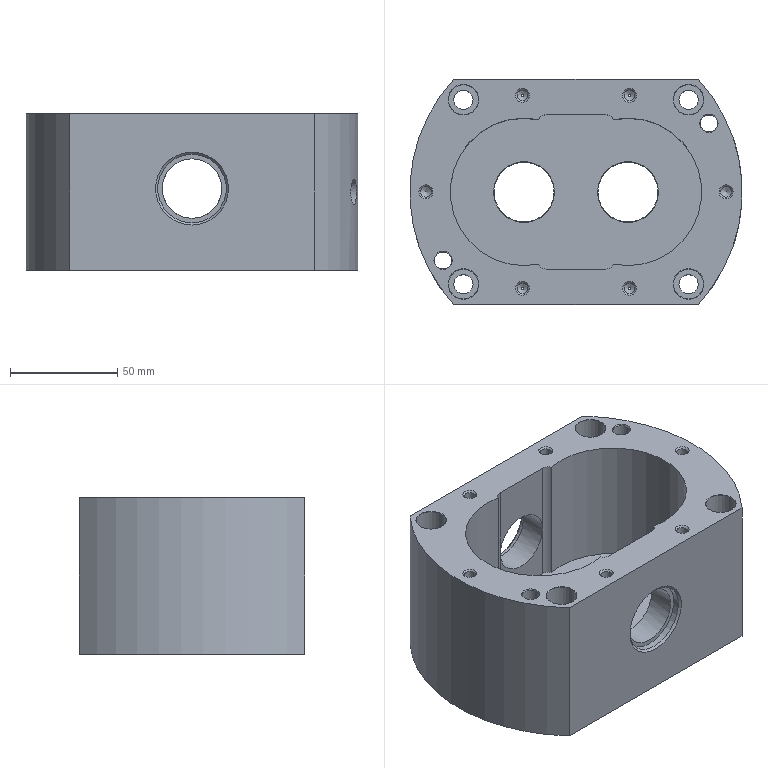NC program | NX | posted with a generic post | part box 155 x 105 x 73.2 mm
Whole program:
N10 G17 G21 G94 G90
(FLOOR_WALL , TOOL : D50)
N12 T02 M6
N14 G54
N16 G17 G0 G90 X-45.316 Y46.597 B0. C0. S1200 M3
N18 G43 Z30. H2
N20 Z2.654
N22 G94 G1 Z-0.346 F1000.
N24 X-42.316
N26 X42.316 F2000.
N28 Y9.999
N30 X-42.316
N32 Y-26.6
N34 X42.316
N36 X45.316
N38 Z2.654
N40 G0 Z30.
N42 X-48.333 Y46.597
N44 Z2.308
N46 G1 Z-0.692 F1000.
N48 X-45.333
N50 X45.333 F2000.
N52 Y9.999
N54 X-45.333
N56 Y-26.6
N58 X45.333
N60 X48.333
N62 Z2.308
N64 G0 Z30.
N66 X-50.64 Y46.597
N68 Z1.962
N70 G1 Z-1.038 F1000.
N72 X-47.64
N74 X47.64 F2000.
N76 Y9.999
N78 X-47.64
N80 Y-26.6
N82 X47.64
N84 X50.64
N86 Z1.962
N88 G0 Z30.
N90 X-52.579 Y46.597
N92 Z1.616
N94 G1 Z-1.384 F1000.
N96 X-49.579
N98 X49.579 F2000.
N100 Y9.999
N102 X-49.579
N104 Y-26.6
N106 X49.579
N108 X52.579
N110 Z1.616
N112 G0 Z30.
N114 X-54.281 Y46.597
N116 Z1.271
N118 G1 Z-1.729 F1000.
N120 X-51.281
N122 X51.281 F2000.
N124 Y9.999
N126 X-51.281
N128 Y-26.6
N130 X51.281
N132 X54.281
N134 Z1.271
N136 G0 Z30.
N138 X-55.815 Y46.597
N140 Z0.925
N142 G1 Z-2.075 F1000.
N144 X-52.815
N146 X52.815 F2000.
N148 Y9.999
N150 X-52.815
N152 Y-26.6
N154 X52.815
N156 X55.815
N158 Z0.925
N160 G0 Z30.
N162 X-57.22 Y46.597
N164 Z0.579
N166 G1 Z-2.421 F1000.
N168 X-54.22
N170 X54.22 F2000.
N172 Y9.999
N174 X-54.22
N176 Y-26.6
N178 X54.22
N180 X57.22
N182 Z0.579
N184 G0 Z30.
N186 X-58.524 Y46.597
N188 Z0.233
N190 G1 Z-2.767 F1000.
N192 X-55.524
N194 X55.524 F2000.
N196 Y9.999
N198 X-55.524
N200 Y-26.6
N202 X55.524
N204 X58.524
N206 Z0.233
N208 G0 Z30.
N210 X-59.744 Y46.597
N212 Z-0.113
N214 G1 Z-3.113 F1000.
N216 X-56.744
N218 X56.744 F2000.
N220 Y9.999
N222 X-56.744
N224 Y-26.6
N226 X56.744
N228 X59.744
N230 Z-0.113
N232 G0 Z30.
N234 X-60.894 Y46.597
N236 Z-0.459
N238 G1 Z-3.459 F1000.
N240 X-57.894
N242 X57.894 F2000.
N244 Y9.999
N246 X-57.894
N248 Y-26.6
N250 X57.894
N252 X60.894
N254 Z-0.459
N256 G0 Z30.
N258 X-61.984 Y46.597
N260 Z-0.804
N262 G1 Z-3.804 F1000.
N264 X-58.984
N266 X58.984 F2000.
N268 Y9.999
N270 X-58.984
N272 Y-26.6
N274 X58.984
N276 X61.984
N278 Z-0.804
N280 G0 Z30.
N282 X-63.021 Y46.597
N284 Z-1.15
N286 G1 Z-4.15 F1000.
N288 X-60.021
N290 X60.021 F2000.
N292 Y9.999
N294 X-60.021
N296 Y-26.6
N298 X60.021
N300 X63.021
N302 Z-1.15
N304 G0 Z30.
N306 X-64.013 Y46.597
N308 Z-1.496
N310 G1 Z-4.496 F1000.
N312 X-61.013
N314 X61.013 F2000.
N316 Y9.999
N318 X-61.013
N320 Y-26.6
N322 X61.013
N324 X64.013
N326 Z-1.496
N328 G0 Z30.
N330 X-64.964 Y46.597
N332 Z-1.842
N334 G1 Z-4.842 F1000.
N336 X-61.964
N338 X61.964 F2000.
N340 Y9.999
N342 X-61.964
N344 Y-26.6
N346 X61.964
N348 X64.964
N350 Z-1.842
N352 G0 Z30.
N354 X-65.878 Y46.597
N356 Z-2.188
N358 G1 Z-5.188 F1000.
N360 X-62.878
N362 X62.878 F2000.
N364 Y9.999
N366 X-62.878
N368 Y-26.6
N370 X62.878
N372 X65.878
N374 Z-2.188
N376 G0 Z30.
N378 X-66.759 Y46.597
N380 Z-2.534
N382 G1 Z-5.534 F1000.
N384 X-63.759
N386 X63.759 F2000.
N388 Y9.999
N390 X-63.759
N392 Y-26.6
N394 X63.759
N396 X66.759
N398 Z-2.534
N400 G0 Z30.
N402 X-67.61 Y46.597
N404 Z-2.879
N406 G1 Z-5.879 F1000.
N408 X-64.61
N410 X64.61 F2000.
N412 Y9.999
N414 X-64.61
N416 Y-26.6
N418 X64.61
N420 X67.61
N422 Z-2.879
N424 G0 Z30.
N426 X-68.433 Y46.597
N428 Z-3.225
N430 G1 Z-6.225 F1000.
N432 X-65.433
N434 X65.433 F2000.
N436 Y9.999
N438 X-65.433
N440 Y-26.6
N442 X65.433
N444 X68.433
N446 Z-3.225
N448 G0 Z30.
N450 X-69.23 Y46.597
N452 Z-3.571
N454 G1 Z-6.571 F1000.
N456 X-66.23
N458 X66.23 F2000.
N460 Y9.999
N462 X-66.23
N464 Y-26.6
N466 X66.23
N468 X69.23
N470 Z-3.571
N472 G0 Z30.
N474 X-70.004 Y46.597
N476 Z-3.917
N478 G1 Z-6.917 F1000.
N480 X-67.004
N482 X67.004 F2000.
N484 Y9.999
N486 X-67.004
N488 Y-26.6
N490 X67.004
N492 X70.004
N494 Z-3.917
N496 G0 Z30.
N498 X-70.756 Y46.597
N500 Z-4.263
N502 G1 Z-7.263 F1000.
N504 X-67.756
N506 X67.756 F2000.
N508 Y9.999
N510 X-67.756
N512 Y-26.6
N514 X67.756
N516 X70.756
N518 Z-4.263
N520 G0 Z30.
N522 X-71.488 Y46.597
N524 Z-4.609
N526 G1 Z-7.609 F1000.
N528 X-68.488
N530 X68.488 F2000.
N532 Y9.999
N534 X-68.488
N536 Y-26.6
N538 X68.488
N540 X71.488
N542 Z-4.609
N544 G0 Z30.
N546 X-72.2 Y46.597
N548 Z-4.954
N550 G1 Z-7.954 F1000.
N552 X-69.2
N554 X69.2 F2000.
N556 Y9.999
N558 X-69.2
N560 Y-26.6
N562 X69.2
N564 X72.2
N566 Z-4.954
N568 G0 Z30.
N570 X-72.895 Y46.597
N572 Z-5.3
N574 G1 Z-8.3 F1000.
N576 X-69.895
N578 X69.895 F2000.
N580 Y9.999
N582 X-69.895
N584 Y-26.6
N586 X69.895
N588 X72.895
N590 Z-5.3
N592 G0 Z30.
N594 X-73.572 Y46.597
N596 Z-5.646
N598 G1 Z-8.646 F1000.
N600 X-70.572
N602 X70.572 F2000.
N604 Y9.999
N606 X-70.572
N608 Y-26.6
N610 X70.572
N612 X73.572
N614 Z-5.646
N616 G0 Z30.
N618 X-74.234 Y46.597
N620 Z-5.992
N622 G1 Z-8.992 F1000.
N624 X-71.234
N626 X71.234 F2000.
N628 Y9.999
N630 X-71.234
N632 Y-26.6
N634 X71.234
N636 X74.234
N638 Z-5.992
N640 G0 Z30.
N642 X-74.88 Y46.597
N644 Z-6.338
N646 G1 Z-9.338 F1000.
N648 X-71.88
N650 X71.88 F2000.
N652 Y9.999
N654 X-71.88
N656 Y-26.6
N658 X71.88
N660 X74.88
N662 Z-6.338
N664 G0 Z30.
N666 X-75.512 Y46.597
N668 Z-6.684
N670 G1 Z-9.684 F1000.
N672 X-72.512
N674 X72.512 F2000.
N676 Y9.999
N678 X-72.512
N680 Y-26.6
N682 X72.512
N684 X75.512
N686 Z-6.684
N688 G0 Z30.
N690 X-76.131 Y46.597
N692 Z-7.029
N694 G1 Z-10.029 F1000.
N696 X-73.131
N698 X73.131 F2000.
N700 Y9.999
N702 X-73.131
N704 Y-26.6
N706 X73.131
N708 X76.131
N710 Z-7.029
N712 G0 Z30.
N714 X-76.736 Y46.597
N716 Z-7.375
N718 G1 Z-10.375 F1000.
N720 X-73.736
N722 X73.736 F2000.
N724 Y9.999
N726 X-73.736
N728 Y-26.6
N730 X73.736
N732 X76.736
N734 Z-7.375
N736 G0 Z30.
N738 X-77.33 Y46.597
N740 Z-7.721
N742 G1 Z-10.721 F1000.
N744 X-74.33
N746 X74.33 F2000.
N748 Y9.999
N750 X-74.33
N752 Y-26.6
N754 X74.33
N756 X77.33
N758 Z-7.721
N760 G0 Z30.
N762 X-77.911 Y46.597
N764 Z-8.067
N766 G1 Z-11.067 F1000.
N768 X-74.911
N770 X74.911 F2000.
N772 Y9.999
N774 X-74.911
N776 Y-26.6
N778 X74.911
N780 X77.911
N782 Z-8.067
N784 G0 Z30.
N786 X-78.481 Y46.597
N788 Z-8.413
N790 G1 Z-11.413 F1000.
N792 X-75.481
N794 X75.481 F2000.
N796 Y9.999
N798 X-75.481
N800 Y-26.6
N802 X75.481
N804 X78.481
N806 Z-8.413
N808 G0 Z30.
N810 X-79.04 Y46.597
N812 Z-8.758
N814 G1 Z-11.758 F1000.
N816 X-76.04
N818 X76.04 F2000.
N820 Y9.999
N822 X-76.04
N824 Y-26.6
N826 X76.04
N828 X79.04
N830 Z-8.758
N832 G0 Z30.
N834 X-79.589 Y46.597
N836 Z-9.104
N838 G1 Z-12.104 F1000.
N840 X-76.589
N842 X76.589 F2000.
N844 Y9.999
N846 X-76.589
N848 Y-26.6
N850 X76.589
N852 X79.589
N854 Z-9.104
N856 G0 Z30.
N858 X-80.128 Y46.597
N860 Z-9.45
N862 G1 Z-12.45 F1000.
N864 X-77.128
N866 X77.128 F2000.
N868 Y9.999
N870 X-77.128
N872 Y-26.6
N874 X77.128
N876 X80.128
N878 Z-9.45
N880 G0 Z30.
N882 X-80.657 Y46.597
N884 Z-9.796
N886 G1 Z-12.796 F1000.
N888 X-77.657
N890 X77.657 F2000.
N892 Y9.999
N894 X-77.657
N896 Y-26.6
N898 X77.657
N900 X80.657
N902 Z-9.796
N904 G0 Z30.
N906 X-81.177 Y46.597
N908 Z-10.142
N910 G1 Z-13.142 F1000.
N912 X-78.177
N914 X78.177 F2000.
N916 Y9.999
N918 X-78.177
N920 Y-26.6
N922 X78.177
N924 X81.177
N926 Z-10.142
N928 G0 Z30.
N930 X-81.688 Y46.597
N932 Z-10.488
N934 G1 Z-13.488 F1000.
N936 X-78.688
N938 X78.688 F2000.
N940 Y9.999
N942 X-78.688
N944 Y-26.6
N946 X78.688
N948 X81.688
N950 Z-10.488
N952 G0 Z30.
N954 X-82.191 Y46.597
N956 Z-10.833
N958 G1 Z-13.833 F1000.
N960 X-79.191
N962 X79.191 F2000.
N964 Y9.999
N966 X-79.191
N968 Y-26.6
N970 X79.191
N972 X82.191
N974 Z-10.833
N976 G0 Z30.
N978 X-82.685 Y46.597
N980 Z-11.179
N982 G1 Z-14.179 F1000.
N984 X-79.685
N986 X79.685 F2000.
N988 Y9.999
N990 X-79.685
N992 Y-26.6
N994 X79.685
N996 X82.685
N998 Z-11.179
N1000 G0 Z30.
N1002 X-83.171 Y46.597
N1004 Z-11.525
N1006 G1 Z-14.525 F1000.
N1008 X-80.171
N1010 X80.171 F2000.
N1012 Y9.999
N1014 X-80.171
N1016 Y-26.6
N1018 X80.171
N1020 X83.171
N1022 Z-11.525
N1024 G0 Z30.
N1026 X-83.649 Y46.597
N1028 Z-11.871
N1030 G1 Z-14.871 F1000.
N1032 X-80.649
N1034 X80.649 F2000.
N1036 Y9.999
N1038 X-80.649
N1040 Y-26.6
N1042 X80.649
N1044 X83.649
N1046 Z-11.871
N1048 G0 Z30.
N1050 X-84.12 Y46.597
N1052 Z-12.217
N1054 G1 Z-15.217 F1000.
N1056 X-81.12
N1058 X81.12 F2000.
N1060 Y9.999
N1062 X-81.12
N1064 Y-26.6
N1066 X81.12
N1068 X84.12
N1070 Z-12.217
N1072 G0 Z30.
N1074 X-84.583 Y46.597
N1076 Z-12.563
N1078 G1 Z-15.563 F1000.
N1080 X-81.583
N1082 X81.583 F2000.
N1084 Y9.999
N1086 X-81.583
N1088 Y-26.6
N1090 X81.583
N1092 X84.583
N1094 Z-12.563
N1096 G0 Z30.
N1098 X-85.04 Y46.597
N1100 Z-12.908
N1102 G1 Z-15.908 F1000.
N1104 X-82.04
N1106 X82.04 F2000.
N1108 Y9.999
N1110 X-82.04
N1112 Y-26.6
N1114 X82.04
N1116 X85.04
N1118 Z-12.908
N1120 G0 Z30.
N1122 X-85.489 Y46.597
N1124 Z-13.254
N1126 G1 Z-16.254 F1000.
N1128 X-82.489
N1130 X82.489 F2000.
N1132 Y9.999
N1134 X-82.489
N1136 Y-26.6
N1138 X82.489
N1140 X85.489
N1142 Z-13.254
N1144 G0 Z30.
N1146 X-85.932 Y46.597
N1148 Z-13.6
N1150 G1 Z-16.6 F1000.
N1152 X-82.932
N1154 X82.932 F2000.
N1156 Y9.999
N1158 X-82.932
N1160 Y-26.6
N1162 X82.932
N1164 X85.932
N1166 Z-13.6
N1168 G0 Z30.
N1170 X-86.368 Y46.597
N1172 Z-13.946
N1174 G1 Z-16.946 F1000.
N1176 X-83.368
N1178 X83.368 F2000.
N1180 Y9.999
N1182 X-83.368
N1184 Y-26.6
N1186 X83.368
N1188 X86.368
N1190 Z-13.946
N1192 G0 Z30.
N1194 X-86.798 Y46.597
N1196 Z-14.292
N1198 G1 Z-17.292 F1000.
N1200 X-83.798
N1202 X83.798 F2000.
N1204 Y9.999
N1206 X-83.798
N1208 Y-26.6
N1210 X83.798
N1212 X86.798
N1214 Z-14.292
N1216 G0 Z30.
N1218 X-87.221 Y46.597
N1220 Z-14.638
N1222 G1 Z-17.638 F1000.
N1224 X-84.221
N1226 X84.221 F2000.
N1228 Y9.999
N1230 X-84.221
N1232 Y-26.6
N1234 X84.221
N1236 X87.221
N1238 Z-14.638
N1240 G0 Z30.
N1242 X-87.639 Y46.597
N1244 Z-14.983
N1246 G1 Z-17.983 F1000.
N1248 X-84.639
N1250 X84.639 F2000.
N1252 Y9.999
N1254 X-84.639
N1256 Y-26.6
N1258 X84.639
N1260 X87.639
N1262 Z-14.983
N1264 G0 Z30.
N1266 X-88.051 Y46.597
N1268 Z-15.329
N1270 G1 Z-18.329 F1000.
N1272 X-85.051
N1274 X85.051 F2000.
N1276 Y9.999
N1278 X-85.051
N1280 Y-26.6
N1282 X85.051
N1284 X88.051
N1286 Z-15.329
N1288 G0 Z30.
N1290 X-88.457 Y46.597
N1292 Z-15.675
N1294 G1 Z-18.675 F1000.
N1296 X-85.457
N1298 X85.457 F2000.
N1300 Y9.999
N1302 X-85.457
N1304 Y-26.6
N1306 X85.457
N1308 X88.457
N1310 Z-15.675
N1312 G0 Z30.
N1314 X-88.857 Y46.597
N1316 Z-16.021
N1318 G1 Z-19.021 F1000.
N1320 X-85.857
N1322 X85.857 F2000.
N1324 Y9.999
N1326 X-85.857
N1328 Y-26.6
N1330 X85.857
N1332 X88.857
N1334 Z-16.021
N1336 G0 Z30.
N1338 X-89.252 Y46.597
N1340 Z-16.367
N1342 G1 Z-19.367 F1000.
N1344 X-86.252
N1346 X86.252 F2000.
N1348 Y9.999
N1350 X-86.252
N1352 Y-26.6
N1354 X86.252
N1356 X89.252
N1358 Z-16.367
N1360 G0 Z30.
N1362 X-89.642 Y46.597
N1364 Z-16.713
N1366 G1 Z-19.713 F1000.
N1368 X-86.642
N1370 X86.642 F2000.
N1372 Y9.999
N1374 X-86.642
N1376 Y-26.6
N1378 X86.642
N1380 X89.642
N1382 Z-16.713
N1384 G0 Z30.
N1386 X-90.026 Y46.597
N1388 Z-17.058
N1390 G1 Z-20.058 F1000.
N1392 X-87.026
N1394 X87.026 F2000.
N1396 Y9.999
N1398 X-87.026
N1400 Y-26.6
N1402 X87.026
N1404 X90.026
N1406 Z-17.058
N1408 G0 Z30.
N1410 X-90.405 Y46.597
N1412 Z-17.404
N1414 G1 Z-20.404 F1000.
N1416 X-87.405
N1418 X87.405 F2000.
N1420 Y9.999
N1422 X-87.405
N1424 Y-26.6
N1426 X87.405
N1428 X90.405
N1430 Z-17.404
N1432 G0 Z30.
N1434 X-90.78 Y46.597
N1436 Z-17.75
N1438 G1 Z-20.75 F1000.
N1440 X-87.78
N1442 X87.78 F2000.
N1444 Y9.999
N1446 X-87.78
N1448 Y-26.6
N1450 X87.78
N1452 X90.78
N1454 Z-17.75
N1456 G0 Z30.
N1458 X-91.149 Y46.597
N1460 Z-18.096
N1462 G1 Z-21.096 F1000.
N1464 X-88.149
N1466 X88.149 F2000.
N1468 Y9.999
N1470 X-88.149
N1472 Y-26.6
N1474 X88.149
N1476 X91.149
N1478 Z-18.096
N1480 G0 Z30.
N1482 X-91.514 Y46.597
N1484 Z-18.442
N1486 G1 Z-21.442 F1000.
N1488 X-88.514
N1490 X88.514 F2000.
N1492 Y9.999
N1494 X-88.514
N1496 Y-26.6
N1498 X88.514
N1500 X91.514
N1502 Z-18.442
N1504 G0 Z30.
N1506 X-91.874 Y46.597
N1508 Z-18.788
N1510 G1 Z-21.788 F1000.
N1512 X-88.874
N1514 X88.874 F2000.
N1516 Y9.999
N1518 X-88.874
N1520 Y-26.6
N1522 X88.874
N1524 X91.874
N1526 Z-18.788
N1528 G0 Z30.
N1530 X-92.229 Y46.597
N1532 Z-19.133
N1534 G1 Z-22.133 F1000.
N1536 X-89.229
N1538 X89.229 F2000.
N1540 Y9.999
N1542 X-89.229
N1544 Y-26.6
N1546 X89.229
N1548 X92.229
N1550 Z-19.133
N1552 G0 Z30.
N1554 X-92.58 Y46.597
N1556 Z-19.479
N1558 G1 Z-22.479 F1000.
N1560 X-89.58
N1562 X89.58 F2000.
N1564 Y9.999
N1566 X-89.58
N1568 Y-26.6
N1570 X89.58
N1572 X92.58
N1574 Z-19.479
N1576 G0 Z30.
N1578 X-92.926 Y46.597
N1580 Z-19.825
N1582 G1 Z-22.825 F1000.
N1584 X-89.926
N1586 X89.926 F2000.
N1588 Y9.999
N1590 X-89.926
N1592 Y-26.6
N1594 X89.926
N1596 X92.926
N1598 Z-19.825
N1600 G0 Z30.
N1602 X-93.268 Y46.597
N1604 Z-20.171
N1606 G1 Z-23.171 F1000.
N1608 X-90.268
N1610 X90.268 F2000.
N1612 Y9.999
N1614 X-90.268
N1616 Y-26.6
N1618 X90.268
N1620 X93.268
N1622 Z-20.171
N1624 G0 Z30.
N1626 X-93.606 Y46.597
N1628 Z-20.517
N1630 G1 Z-23.517 F1000.
N1632 X-90.606
N1634 X90.606 F2000.
N1636 Y9.999
N1638 X-90.606
N1640 Y-26.6
N1642 X90.606
N1644 X93.606
N1646 Z-20.517
N1648 G0 Z30.
N1650 X-93.94 Y46.597
N1652 Z-20.863
N1654 G1 Z-23.863 F1000.
N1656 X-90.94
N1658 X90.94 F2000.
N1660 Y9.999
N1662 X-90.94
N1664 Y-26.6
N1666 X90.94
N1668 X93.94
N1670 Z-20.863
N1672 G0 Z30.
N1674 X-94.269 Y46.597
N1676 Z-21.208
N1678 G1 Z-24.208 F1000.
N1680 X-91.269
N1682 X91.269 F2000.
N1684 Y9.999
N1686 X-91.269
N1688 Y-26.6
N1690 X91.269
N1692 X94.269
N1694 Z-21.208
N1696 G0 Z30.
N1698 X-94.595 Y46.597
N1700 Z-21.554
N1702 G1 Z-24.554 F1000.
N1704 X-91.595
N1706 X91.595 F2000.
N1708 Y9.999
N1710 X-91.595
N1712 Y-26.6
N1714 X91.595
N1716 X94.595
N1718 Z-21.554
N1720 G0 Z30.
N1722 X-94.917 Y46.597
N1724 Z-21.9
N1726 G1 Z-24.9 F1000.
N1728 X-91.917
N1730 X91.917 F2000.
N1732 Y9.999
N1734 X-91.917
N1736 Y-26.6
N1738 X91.917
N1740 X94.917
N1742 Z-21.9
N1744 G0 Z30.
(FLOOR_WALL_COPY , TOOL : D50)
N1746 X-95.009 Y46.597 S2500
N1748 Z-22.
N1750 G1 Z-25. F1000.
N1752 X-92.009
N1754 X92.009
N1756 Y9.999
N1758 X-92.009
N1760 Y-26.6
N1762 X92.009
N1764 X95.009
N1766 Z-22.
N1768 G0 Z30.
N1770 M5
(HOLE_MILLING , TOOL : D10)
N1772 T10 M6
N1774 G54
N1776 G17 G0 G90 X0. Y-1.6 B0. C0. S3000 M3
N1778 G43 Z30. H10
N1780 Z-24.5
N1782 G94 G3 X-1.25 Y-0.35 R1.25 F2200.
N1784 X-2.5 Y-1.6 R1.25
N1786 X-2.5 Y-1.6 Z-24.72 I2.5 J0.
N1788 X-2.5 Y-1.6 Z-24.94 I2.5 J0.
N1790 X-2.5 Y-1.6 Z-25.16 I2.5 J0.
N1792 X-2.5 Y-1.6 Z-25.38 I2.5 J0.
N1794 X-2.5 Y-1.6 Z-25.6 I2.5 J0.
N1796 X-2.5 Y-1.6 Z-25.82 I2.5 J0.
N1798 X-2.5 Y-1.6 Z-26.04 I2.5 J0.
N1800 X-2.5 Y-1.6 Z-26.26 I2.5 J0.
N1802 X-2.5 Y-1.6 Z-26.48 I2.5 J0.
N1804 X-2.5 Y-1.6 Z-26.7 I2.5 J0.
N1806 X-2.5 Y-1.6 Z-26.92 I2.5 J0.
N1808 X-2.5 Y-1.6 Z-27.14 I2.5 J0.
N1810 X-2.5 Y-1.6 Z-27.36 I2.5 J0.
N1812 X-2.5 Y-1.6 Z-27.58 I2.5 J0.
N1814 X-2.5 Y-1.6 Z-27.8 I2.5 J0.
N1816 X-2.5 Y-1.6 Z-28.02 I2.5 J0.
N1818 X-2.5 Y-1.6 Z-28.24 I2.5 J0.
N1820 X-2.5 Y-1.6 Z-28.46 I2.5 J0.
N1822 X-2.5 Y-1.6 Z-28.68 I2.5 J0.
N1824 X-2.5 Y-1.6 Z-28.9 I2.5 J0.
N1826 X2.399 Y-2.304 Z-29. R2.5
N1828 X0.711 Y0.836 R2.538
N1830 X-2.483 Y-0.8 R2.572
N1832 X-0.863 Y-4.12 R2.629
N1834 X2.565 Y-2.5 R2.698
N1836 X0.966 Y0.999 R2.738
N1838 X-2.643 Y-0.595 R2.807
N1840 X-1.073 Y-4.274 R2.847
N1842 X2.716 Y-2.715 R2.916
N1844 X1.185 Y1.146 R2.956
N1846 X-2.786 Y-0.371 R3.025
N1848 X-1.301 Y-4.414 R3.065
N1850 X2.852 Y-2.948 R3.135
N1852 X1.422 Y1.277 R3.174
N1854 X-2.914 Y-0.13 R3.244
N1856 X-1.546 Y-4.536 R3.283
N1858 X2.971 Y-3.197 R3.353
N1860 X1.675 Y1.39 R3.392
N1862 X-3.023 Y0.128 R3.462
N1864 X-1.807 Y-4.64 R3.501
N1866 X3.07 Y-3.462 R3.571
N1868 X1.943 Y1.484 R3.611
N1870 X-3.113 Y0.4 R3.68
N1872 X-2.083 Y-4.724 R3.72
N1874 X3.15 Y-3.742 R3.789
N1876 X2.226 Y1.558 R3.829
N1878 X-3.182 Y0.687 R3.898
N1880 X-2.372 Y-4.787 R3.938
N1882 X3.208 Y-4.034 R4.007
N1884 X2.521 Y1.61 R4.047
N1886 X-3.229 Y0.985 R4.116
N1888 X-2.673 Y-4.828 R4.156
N1890 X3.244 Y-4.338 R4.226
N1892 X2.827 Y1.64 R4.265
N1894 X-3.254 Y1.294 R4.335
N1896 X-2.984 Y-4.846 R4.374
N1898 X3.257 Y-4.652 R4.444
N1900 X3.143 Y1.646 R4.483
N1902 X-3.254 Y1.612 R4.553
N1904 X-3.303 Y-4.84 R4.592
N1906 X3.245 Y-4.974 R4.662
N1908 X3.466 Y1.628 R4.701
N1910 X-3.23 Y1.938 R4.771
N1912 X-3.63 Y-4.809 R4.811
N1914 X3.209 Y-5.303 R4.88
N1916 X3.796 Y1.584 R4.92
N1918 X-3.181 Y2.27 R4.989
N1920 X-3.962 Y-4.753 R5.029
N1922 X3.146 Y-5.637 R5.098
N1924 X4.13 Y1.515 R5.138
N1926 X-3.105 Y2.605 R5.207
N1928 X-4.298 Y-4.67 R5.247
N1930 X3.058 Y-5.974 R5.316
N1932 X4.466 Y1.419 R5.356
N1934 X-3.003 Y2.942 R5.426
N1936 X-4.635 Y-4.561 R5.465
N1938 X2.942 Y-6.311 R5.535
N1940 X4.803 Y1.296 R5.574
N1942 X-2.874 Y3.28 R5.644
N1944 X-4.972 Y-4.425 R5.683
N1946 X2.799 Y-6.649 R5.753
N1948 X5.139 Y1.146 R5.792
N1950 X-2.718 Y3.616 R5.862
N1952 X-5.306 Y-4.261 R5.902
N1954 X2.629 Y-6.983 R5.971
N1956 X5.472 Y0.969 R6.011
N1958 X-2.534 Y3.949 R6.08
N1960 X-5.637 Y-4.07 R6.12
N1962 X2.432 Y-7.313 R6.189
N1964 X5.8 Y0.764 R6.229
N1966 X-2.323 Y4.276 R6.298
N1968 X-5.962 Y-3.852 R6.338
N1970 X2.207 Y-7.636 R6.407
N1972 X6.121 Y0.533 R6.447
N1974 X-2.084 Y4.595 R6.516
N1976 X-6.278 Y-3.606 R6.556
N1978 X1.955 Y-7.951 R6.626
N1980 X6.433 Y0.273 R6.665
N1982 X-1.819 Y4.905 R6.735
N1984 X-6.585 Y-3.334 R6.774
N1986 X1.676 Y-8.256 R6.844
N1988 X6.734 Y-0.012 R6.883
N1990 X-1.526 Y5.204 R6.953
N1992 X-6.879 Y-3.035 R6.992
N1994 X1.37 Y-8.548 R7.062
N1996 X7.021 Y-0.325 R7.102
N1998 X-1.208 Y5.489 R7.171
N2000 X-7.16 Y-2.71 R7.211
N2002 X1.039 Y-8.826 R7.28
N2004 X7.295 Y-0.663 R7.32
N2006 X-0.864 Y5.759 R7.389
N2008 X-7.425 Y-2.359 R7.429
N2010 X0.682 Y-9.087 R7.498
N2012 X7.551 Y-1.025 R7.538
N2014 X-0.495 Y6.011 R7.607
N2016 X-7.672 Y-1.984 R7.647
N2018 X0.301 Y-9.33 R7.716
N2020 X7.789 Y-1.413 R7.756
N2022 X-0.102 Y6.245 R7.826
N2024 X-7.9 Y-1.585 R7.865
N2026 X-0.103 Y-9.554 R7.935
N2028 X8.006 Y-1.823 R7.974
N2030 X0.314 Y6.458 R8.044
N2032 X-8.106 Y-1.164 R8.083
N2034 X-0.53 Y-9.756 R8.153
N2036 X8.201 Y-2.255 R8.192
N2038 X0.752 Y6.648 R8.262
N2040 X-8.29 Y-0.721 R8.302
N2042 X-0.978 Y-9.934 R8.371
N2044 X8.372 Y-2.708 R8.411
N2046 X1.21 Y6.813 R8.48
N2048 X-8.449 Y-0.258 R8.52
N2050 X-1.446 Y-10.087 R8.589
N2052 X8.518 Y-3.18 R8.629
N2054 X1.687 Y6.953 R8.698
N2056 X-8.581 Y0.224 R8.738
N2058 X-1.932 Y-10.213 R8.807
N2060 X8.637 Y-3.671 R8.847
N2062 X2.182 Y7.066 R8.917
N2064 X-8.686 Y0.722 R8.956
N2066 X-2.436 Y-10.311 R9.026
N2068 X8.727 Y-4.178 R9.065
N2070 X2.693 Y7.15 R9.135
N2072 X-8.761 Y1.237 R9.174
N2074 X-2.954 Y-10.38 R9.244
N2076 X8.787 Y-4.7 R9.283
N2078 X3.218 Y7.203 R9.353
N2080 X-8.806 Y1.766 R9.392
N2082 X-3.486 Y-10.418 R9.462
N2084 X8.817 Y-5.234 R9.502
N2086 X3.756 Y7.225 R9.571
N2088 X-8.819 Y2.306 R9.611
N2090 X-4.03 Y-10.423 R9.68
N2092 X8.813 Y-5.78 R9.72
N2094 X4.305 Y7.214 R9.789
N2096 X-8.799 Y2.857 R9.829
N2098 X-4.583 Y-10.396 R9.898
N2100 X8.777 Y-6.335 R9.938
N2102 X4.863 Y7.169 R10.007
N2104 X-8.745 Y3.416 R10.047
N2106 X-5.144 Y-10.334 R10.117
N2108 X8.706 Y-6.898 R10.156
N2110 X5.427 Y7.09 R10.226
N2112 X-8.657 Y3.981 R10.265
N2114 X-5.711 Y-10.237 R10.335
N2116 X8.599 Y-7.465 R10.374
N2118 X5.996 Y6.976 R10.444
N2120 X-8.533 Y4.55 R10.483
N2122 X-6.281 Y-10.105 R10.553
N2124 X8.457 Y-8.036 R10.592
N2126 X6.567 Y6.825 R10.662
N2128 X-8.372 Y5.121 R10.702
N2130 X-6.852 Y-9.936 R10.771
N2132 X8.325 Y-8.578 R10.828
N2134 X7.138 Y6.638 R10.862
N2136 X-8.238 Y5.538 R10.9
N2138 X7.138 Y6.638 R-10.9
N2140 X-0.55 Y6.088 R5.45
N2142 X0. Y-1.6 R5.45
N2144 G0 Z30.
(HOLE_MILLING_COPY , TOOL : D10)
N2146 Z-28.5
N2148 G3 X-1.25 Y-0.35 R1.25
N2150 X-2.5 Y-1.6 R1.25
N2152 X-2.5 Y-1.6 Z-28.72 I2.5 J0.
N2154 X-2.5 Y-1.6 Z-28.94 I2.5 J0.
N2156 X-2.5 Y-1.6 Z-29.16 I2.5 J0.
N2158 X-2.5 Y-1.6 Z-29.38 I2.5 J0.
N2160 X-2.5 Y-1.6 Z-29.6 I2.5 J0.
N2162 X-2.5 Y-1.6 Z-29.82 I2.5 J0.
N2164 X-2.5 Y-1.6 Z-30.04 I2.5 J0.
N2166 X-2.5 Y-1.6 Z-30.26 I2.5 J0.
N2168 X-2.5 Y-1.6 Z-30.48 I2.5 J0.
N2170 X-2.5 Y-1.6 Z-30.7 I2.5 J0.
N2172 X-2.5 Y-1.6 Z-30.92 I2.5 J0.
N2174 X-2.5 Y-1.6 Z-31.14 I2.5 J0.
N2176 X-2.5 Y-1.6 Z-31.36 I2.5 J0.
N2178 X-2.5 Y-1.6 Z-31.58 I2.5 J0.
N2180 X-2.5 Y-1.6 Z-31.8 I2.5 J0.
N2182 X-2.5 Y-1.6 Z-32.02 I2.5 J0.
N2184 X-2.5 Y-1.6 Z-32.24 I2.5 J0.
N2186 X-2.5 Y-1.6 Z-32.46 I2.5 J0.
N2188 X-2.5 Y-1.6 Z-32.68 I2.5 J0.
N2190 X-2.5 Y-1.6 Z-32.9 I2.5 J0.
N2192 X-2.5 Y-1.6 Z-33.12 I2.5 J0.
N2194 X-2.5 Y-1.6 Z-33.34 I2.5 J0.
N2196 X-2.5 Y-1.6 Z-33.56 I2.5 J0.
N2198 X-2.5 Y-1.6 Z-33.78 I2.5 J0.
N2200 X-2.5 Y-1.6 Z-34. I2.5 J0.
N2202 X-2.5 Y-1.6 Z-34.22 I2.5 J0.
N2204 X-2.5 Y-1.6 Z-34.44 I2.5 J0.
N2206 X-2.5 Y-1.6 Z-34.66 I2.5 J0.
N2208 X-2.5 Y-1.6 Z-34.88 I2.5 J0.
N2210 X-2.5 Y-1.6 Z-35.1 I2.5 J0.
N2212 X-2.5 Y-1.6 Z-35.32 I2.5 J0.
N2214 X-2.5 Y-1.6 Z-35.54 I2.5 J0.
N2216 X-2.5 Y-1.6 Z-35.76 I2.5 J0.
N2218 X-2.5 Y-1.6 Z-35.98 I2.5 J0.
N2220 X-2.5 Y-1.6 Z-36.2 I2.5 J0.
N2222 X-2.5 Y-1.6 Z-36.42 I2.5 J0.
N2224 X-2.5 Y-1.6 Z-36.64 I2.5 J0.
N2226 X-2.5 Y-1.6 Z-36.86 I2.5 J0.
N2228 X-2.5 Y-1.6 Z-37.08 I2.5 J0.
N2230 X-2.5 Y-1.6 Z-37.3 I2.5 J0.
N2232 X-2.5 Y-1.6 Z-37.52 I2.5 J0.
N2234 X-2.5 Y-1.6 Z-37.74 I2.5 J0.
N2236 X-2.5 Y-1.6 Z-37.96 I2.5 J0.
N2238 X-2.5 Y-1.6 Z-38.18 I2.5 J0.
N2240 X-2.5 Y-1.6 Z-38.4 I2.5 J0.
N2242 X-2.5 Y-1.6 Z-38.62 I2.5 J0.
N2244 X-2.5 Y-1.6 Z-38.84 I2.5 J0.
N2246 X-2.5 Y-1.6 Z-39.06 I2.5 J0.
N2248 X-2.5 Y-1.6 Z-39.28 I2.5 J0.
N2250 X-2.5 Y-1.6 Z-39.5 I2.5 J0.
N2252 X-2.5 Y-1.6 Z-39.72 I2.5 J0.
N2254 X-2.5 Y-1.6 Z-39.94 I2.5 J0.
N2256 X-2.5 Y-1.6 Z-40.16 I2.5 J0.
N2258 X-2.5 Y-1.6 Z-40.38 I2.5 J0.
N2260 X-2.5 Y-1.6 Z-40.6 I2.5 J0.
N2262 X-2.5 Y-1.6 Z-40.82 I2.5 J0.
N2264 X-2.5 Y-1.6 Z-41.04 I2.5 J0.
N2266 X-2.5 Y-1.6 Z-41.26 I2.5 J0.
N2268 X-2.5 Y-1.6 Z-41.48 I2.5 J0.
N2270 X-2.5 Y-1.6 Z-41.7 I2.5 J0.
N2272 X-2.5 Y-1.6 Z-41.92 I2.5 J0.
N2274 X1.637 Y-3.489 Z-42. R2.5
N2276 X1.893 Y0.086 R2.534
N2278 X-1.703 Y0.365 R2.566
N2280 X-2.012 Y-3.325 R2.618
N2282 X1.768 Y-3.641 R2.682
N2284 X2.087 Y0.19 R2.718
N2286 X-1.834 Y0.516 R2.782
N2288 X-2.163 Y-3.456 R2.818
N2290 X1.899 Y-3.792 R2.882
N2292 X2.238 Y0.321 R2.918
N2294 X-1.965 Y0.667 R2.982
N2296 X-2.314 Y-3.587 R3.018
N2298 X2.03 Y-3.943 R3.082
N2300 X2.389 Y0.452 R3.118
N2302 X-2.096 Y0.818 R3.182
N2304 X-2.465 Y-3.718 R3.218
N2306 X2.161 Y-4.094 R3.282
N2308 X2.541 Y0.583 R3.318
N2310 X-2.227 Y0.97 R3.382
N2312 X-2.616 Y-3.849 R3.418
N2314 X2.292 Y-4.245 R3.482
N2316 X2.692 Y0.714 R3.518
N2318 X-2.357 Y1.121 R3.582
N2320 X-2.767 Y-3.98 R3.618
N2322 X2.423 Y-4.396 R3.682
N2324 X2.843 Y0.845 R3.718
N2326 X-2.488 Y1.272 R3.782
N2328 X-2.919 Y-4.111 R3.818
N2330 X2.554 Y-4.547 R3.882
N2332 X2.994 Y0.976 R3.918
N2334 X-2.619 Y1.423 R3.982
N2336 X-3.07 Y-4.242 R4.018
N2338 X2.685 Y-4.699 R4.082
N2340 X3.145 Y1.107 R4.118
N2342 X-2.75 Y1.574 R4.182
N2344 X-3.221 Y-4.373 R4.218
N2346 X2.816 Y-4.85 R4.282
N2348 X3.296 Y1.238 R4.318
N2350 X-2.881 Y1.725 R4.382
N2352 X-3.372 Y-4.504 R4.418
N2354 X2.947 Y-5.001 R4.482
N2356 X3.448 Y1.369 R4.518
N2358 X-3.012 Y1.876 R4.582
N2360 X-3.523 Y-4.635 R4.618
N2362 X3.078 Y-5.152 R4.682
N2364 X3.599 Y1.5 R4.718
N2366 X-3.143 Y2.028 R4.782
N2368 X-3.674 Y-4.766 R4.818
N2370 X3.209 Y-5.303 R4.882
N2372 X3.75 Y1.631 R4.918
N2374 X-3.274 Y2.179 R4.982
N2376 X-3.825 Y-4.897 R5.018
N2378 X3.34 Y-5.454 R5.082
N2380 X3.901 Y1.762 R5.118
N2382 X-3.405 Y2.33 R5.182
N2384 X-3.977 Y-5.028 R5.218
N2386 X3.471 Y-5.605 R5.282
N2388 X4.052 Y1.893 R5.318
N2390 X-3.536 Y2.481 R5.382
N2392 X-4.128 Y-5.159 R5.418
N2394 X3.602 Y-5.757 R5.482
N2396 X4.203 Y2.024 R5.518
N2398 X-3.667 Y2.632 R5.582
N2400 X-4.279 Y-5.29 R5.618
N2402 X3.733 Y-5.908 R5.682
N2404 X4.354 Y2.155 R5.718
N2406 X-3.798 Y2.783 R5.782
N2408 X-4.43 Y-5.421 R5.818
N2410 X3.864 Y-6.059 R5.882
N2412 X4.506 Y2.286 R5.918
N2414 X-3.929 Y2.934 R5.982
N2416 X-4.581 Y-5.552 R6.018
N2418 X3.995 Y-6.21 R6.082
N2420 X4.657 Y2.417 R6.118
N2422 X-4.06 Y3.086 R6.182
N2424 X-4.732 Y-5.683 R6.218
N2426 X4.126 Y-6.361 R6.282
N2428 X4.808 Y2.548 R6.318
N2430 X-4.191 Y3.237 R6.382
N2432 X-4.883 Y-5.813 R6.418
N2434 X4.257 Y-6.512 R6.482
N2436 X4.959 Y2.679 R6.518
N2438 X-4.322 Y3.388 R6.582
N2440 X-5.035 Y-5.944 R6.618
N2442 X4.388 Y-6.664 R6.682
N2444 X5.11 Y2.81 R6.718
N2446 X-4.453 Y3.539 R6.782
N2448 X-5.186 Y-6.075 R6.818
N2450 X4.519 Y-6.815 R6.882
N2452 X5.261 Y2.941 R6.918
N2454 X-4.584 Y3.69 R6.982
N2456 X-5.337 Y-6.206 R7.018
N2458 X4.65 Y-6.966 R7.082
N2460 X5.413 Y3.072 R7.118
N2462 X-4.715 Y3.841 R7.182
N2464 X-5.488 Y-6.337 R7.218
N2466 X4.78 Y-7.117 R7.282
N2468 X5.564 Y3.203 R7.318
N2470 X-4.846 Y3.993 R7.382
N2472 X-5.639 Y-6.468 R7.418
N2474 X4.911 Y-7.268 R7.482
N2476 X5.715 Y3.334 R7.518
N2478 X-4.977 Y4.144 R7.582
N2480 X-5.79 Y-6.599 R7.618
N2482 X5.042 Y-7.419 R7.682
N2484 X5.866 Y3.465 R7.718
N2486 X-5.108 Y4.295 R7.782
N2488 X-5.942 Y-6.73 R7.818
N2490 X5.173 Y-7.57 R7.882
N2492 X6.017 Y3.596 R7.918
N2494 X-5.239 Y4.446 R7.982
N2496 X-6.093 Y-6.861 R8.018
N2498 X5.304 Y-7.722 R8.082
N2500 X6.168 Y3.727 R8.118
N2502 X-5.37 Y4.597 R8.182
N2504 X-6.244 Y-6.992 R8.218
N2506 X5.435 Y-7.873 R8.282
N2508 X6.319 Y3.858 R8.318
N2510 X-5.501 Y4.748 R8.382
N2512 X-6.395 Y-7.123 R8.418
N2514 X5.566 Y-8.024 R8.482
N2516 X6.471 Y3.989 R8.518
N2518 X-5.632 Y4.899 R8.582
N2520 X-6.546 Y-7.254 R8.618
N2522 X5.697 Y-8.175 R8.682
N2524 X6.603 Y4.166 R8.734
N2526 X-5.763 Y5.051 R8.766
N2528 X-6.651 Y-7.363 R8.8
N2530 X-5.763 Y5.051 R-8.8
N2532 X-6.207 Y-1.156 R4.4
N2534 X0. Y-1.6 R4.4
N2536 G0 Z30.
N2538 M5
(HOLE_MILLING_COPY_1 , TOOL : D10JING)
N2540 T11 M6
N2542 G54
N2544 G17 G0 G90 X0. Y-1.6 B0. C0. S5000 M3
N2546 G43 Z30. H11
N2548 Z-29.
N2550 G94 G1 X-7.486 Y0.924 F1000.
N2552 G3 X-11. Y-1.6 R2.663
N2554 X0. Y-12.6 R11.
N2556 X-11. Y-1.6 R-11.
N2558 X-7.486 Y-4.124 R2.663
N2560 G1 X0. Y-1.6
N2562 G0 Z30.
(HOLE_MILLING_COPY_1_COPY , TOOL : D10JING)
N2564 Z-42.
N2566 G3 X-4.45 Y2.85 R4.45
N2568 X-8.9 Y-1.6 R4.45
N2570 X0. Y-10.5 R8.9
N2572 X-8.9 Y-1.6 R-8.9
N2574 X-4.45 Y-6.05 R4.45
N2576 X0. Y-1.6 R4.45
N2578 G0 Z30.
N2580 M5
(PLANAR_MILL , TOOL : D6A45)
N2582 T07 M6
N2584 G54
N2586 G17 G0 G90 X-1.546 Y-15.313 B0. C0. S7500 M3
N2588 G43 Z30. H7
N2590 Z-23.5
N2592 G94 G1 Z-26.5 F1250.
N2594 X-0.766 Y-16.243
N2596 G3 X0. Y-16.6 R1.
N2598 X15. Y-1.6 R15.
N2600 X0. Y-16.6 R-15.
N2602 X0.766 Y-16.243 R1.
N2604 G1 X-0.766 Y-16.743
N2606 G3 X0. Y-17.1 R1.
N2608 X15.5 Y-1.6 R15.5
N2610 X0. Y-17.1 R-15.5
N2612 X0.766 Y-16.743 R1.
N2614 G1 X1.543 Y-15.816
N2616 Z-23.5
N2618 G0 Z30.
(PLANAR_MILL_COPY , TOOL : D6A45)
N2620 X-58.482 Y39.7
N2622 Z-24.
N2624 G1 Z-27.
N2626 X-57.775 Y38.857
N2628 G3 X-57.009 Y38.5 R1.
N2630 G1 X57.009
N2632 G3 X57.775 Y38.857 R1.
N2634 G1 X58.482 Y39.7
N2636 Z-24.
N2638 G0 Z30.
N2640 Y-39.7
N2642 Z-24.
N2644 G1 Z-27.
N2646 X57.775 Y-38.857
N2648 G3 X57.009 Y-38.5 R1.
N2650 G1 X-57.009
N2652 G3 X-57.775 Y-38.857 R1.
N2654 G1 X-58.482 Y-39.7
N2656 Z-24.
N2658 G0 Z30.
N2660 M5
N2662 M2